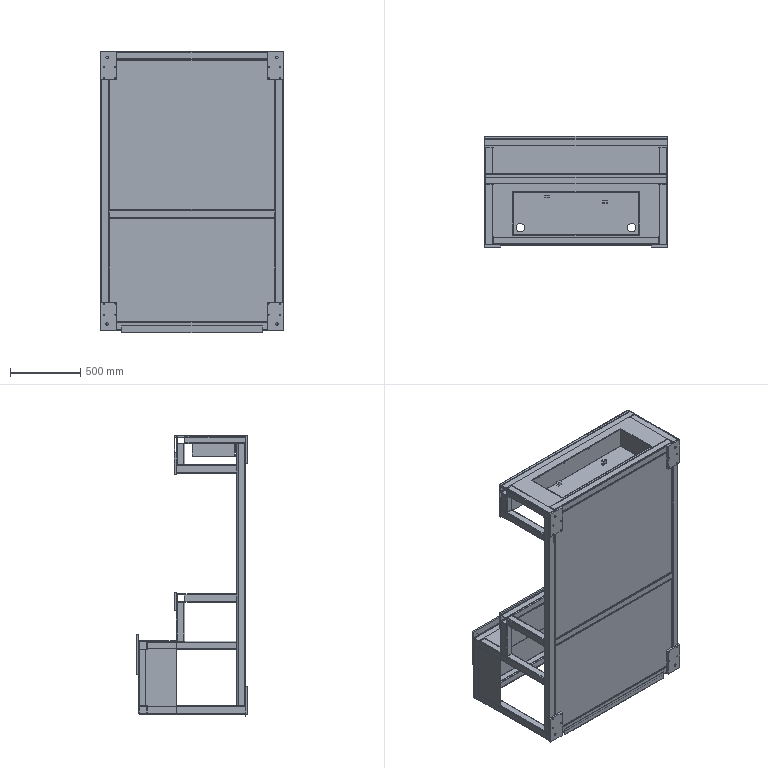Part | NX | features BREP 35 | 35 solids | 1036 faces | box 1303 x 790 x 2009 mm | volume 36444452 mm3 | cylinder 500 | plane 488 | spline 28 | cone 20 | commonest cylinder face diameters 8 x106 16 x100 5 x56 8.5 x56 6.8 x54 3.3 x38